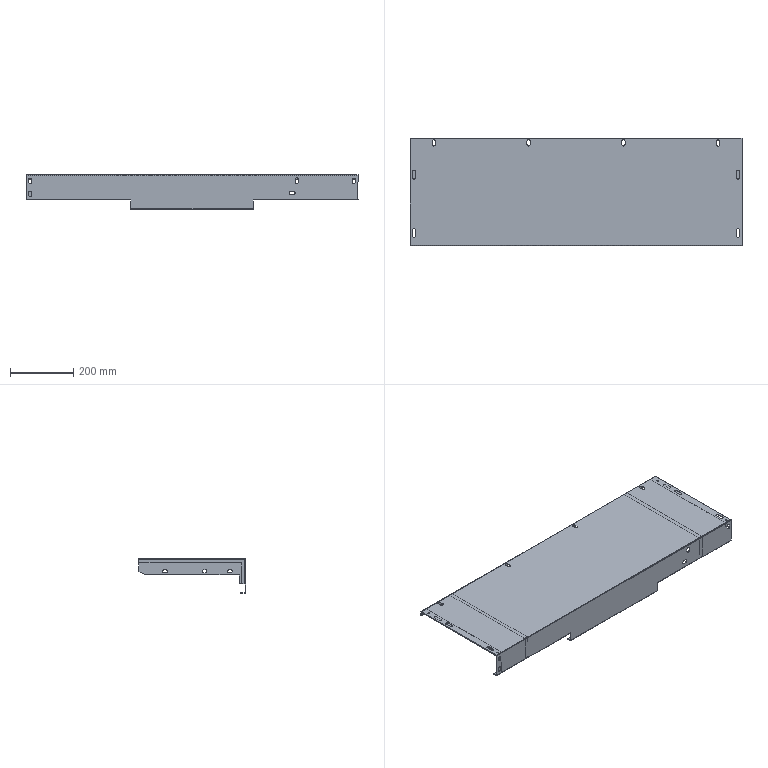Part | SolidWorks | features MirrorCompFeat 2, ReferencePattern 2 | 5 solids | 305 faces | box 1050 x 339.5 x 110 mm | volume 828288 mm3 | plane 212 | cylinder 93 | commonest cylinder face diameters 10 x34 9 x20 6 x12 0.4 x9 3.4 x5 11 x5